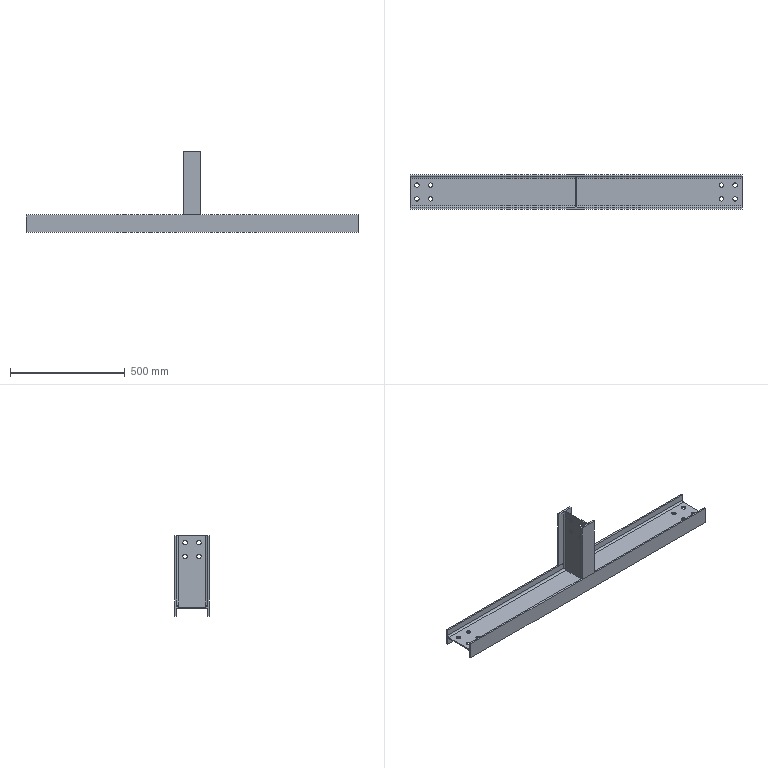Part | STEP file | Mirror_粉仓辅梁4主体1_Default<As Machined> | 2 solids | 66 faces | box 1445 x 150 x 350 mm | volume 3078143 mm3 | plane 34 | cylinder 32 | commonest cylinder face diameters 19 x24 16 x8